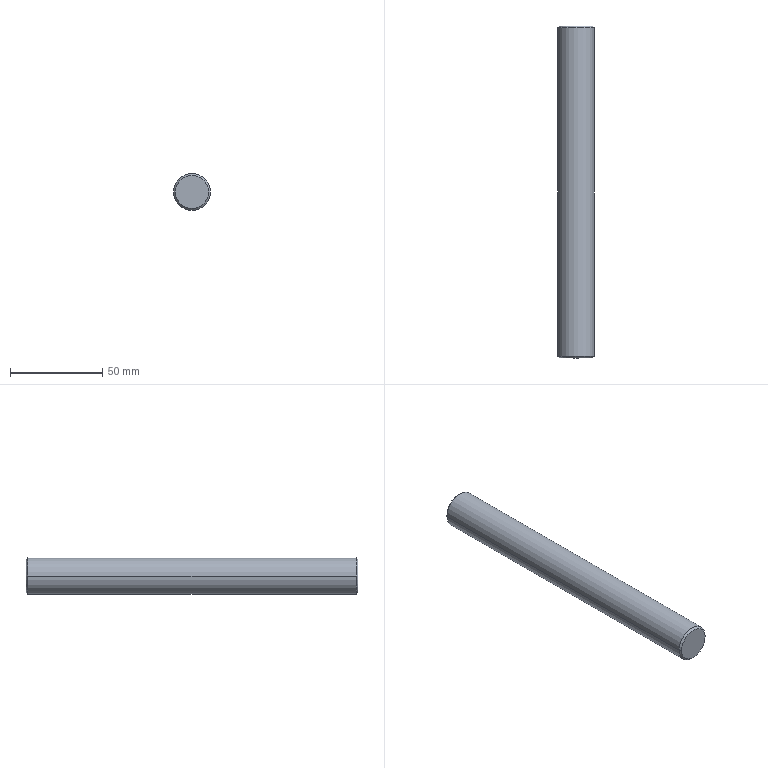Part | SolidWorks | features BaseBody 1 | 1 solid | 8 faces | box 20 x 180 x 20 mm | volume 56488 mm3 | cone 4 | cylinder 2 | plane 2 | commonest cylinder face diameters 20 x2
STEP:
#1=CARTESIAN_POINT('',(-9.,90.,0.));
#2=VERTEX_POINT('',#1);
#3=CARTESIAN_POINT('',(9.,90.,0.));
#4=VERTEX_POINT('',#3);
#5=CARTESIAN_POINT('',(0.,90.,0.));
#6=DIRECTION('',(0.,1.,0.));
#7=DIRECTION('',(-1.,0.,0.));
#8=AXIS2_PLACEMENT_3D('',#5,#6,#7);
#9=CIRCLE('',#8,9.);
#10=EDGE_CURVE('',#2,#4,#9,.T.);
#11=ORIENTED_EDGE('',*,*,#10,.F.);
#12=CARTESIAN_POINT('',(-10.,89.,0.));
#13=VERTEX_POINT('',#12);
#14=CARTESIAN_POINT('',(-10.,89.,0.));
#15=DIRECTION('',(-0.7071,-0.7071,0.));
#16=VECTOR('',#15,1000.);
#17=LINE('',#14,#16);
#18=EDGE_CURVE('',#2,#13,#17,.T.);
#19=ORIENTED_EDGE('',*,*,#18,.T.);
#20=CARTESIAN_POINT('',(10.,89.,0.));
#21=VERTEX_POINT('',#20);
#22=CARTESIAN_POINT('',(0.,89.,0.));
#23=DIRECTION('',(0.,1.,0.));
#24=DIRECTION('',(-1.,0.,0.));
#25=AXIS2_PLACEMENT_3D('',#22,#23,#24);
#26=CIRCLE('',#25,10.);
#27=EDGE_CURVE('',#13,#21,#26,.T.);
#28=ORIENTED_EDGE('',*,*,#27,.T.);
#29=CARTESIAN_POINT('',(10.,89.,0.));
#30=DIRECTION('',(0.7071,-0.7071,0.));
#31=VECTOR('',#30,1000.);
#32=LINE('',#29,#31);
#33=EDGE_CURVE('',#4,#21,#32,.T.);
#34=ORIENTED_EDGE('',*,*,#33,.F.);
#35=EDGE_LOOP('',(#11,#19,#28,#34));
#36=FACE_OUTER_BOUND('',#35,.T.);
#37=CARTESIAN_POINT('',(0.,89.,0.));
#38=DIRECTION('',(0.,-1.,0.));
#39=DIRECTION('',(1.,0.,0.));
#40=AXIS2_PLACEMENT_3D('',#37,#38,#39);
#41=CONICAL_SURFACE('',#40,10.,0.7854);
#42=ADVANCED_FACE('',(#36),#41,.T.);
#43=CARTESIAN_POINT('',(-10.,-89.,0.));
#44=VERTEX_POINT('',#43);
#45=CARTESIAN_POINT('',(10.,-89.,0.));
#46=VERTEX_POINT('',#45);
#47=CARTESIAN_POINT('',(0.,-89.,0.));
#48=DIRECTION('',(0.,1.,0.));
#49=DIRECTION('',(-1.,0.,0.));
#50=AXIS2_PLACEMENT_3D('',#47,#48,#49);
#51=CIRCLE('',#50,10.);
#52=EDGE_CURVE('',#44,#46,#51,.T.);
#53=ORIENTED_EDGE('',*,*,#52,.T.);
#54=CARTESIAN_POINT('',(10.,90.,0.));
#55=DIRECTION('',(0.,1.,0.));
#56=VECTOR('',#55,1000.);
#57=LINE('',#54,#56);
#58=EDGE_CURVE('',#46,#21,#57,.T.);
#59=ORIENTED_EDGE('',*,*,#58,.T.);
#60=ORIENTED_EDGE('',*,*,#27,.F.);
#61=CARTESIAN_POINT('',(-10.,90.,0.));
#62=DIRECTION('',(0.,1.,0.));
#63=VECTOR('',#62,1000.);
#64=LINE('',#61,#63);
#65=EDGE_CURVE('',#44,#13,#64,.T.);
#66=ORIENTED_EDGE('',*,*,#65,.F.);
#67=EDGE_LOOP('',(#53,#59,#60,#66));
#68=FACE_OUTER_BOUND('',#67,.T.);
#69=CARTESIAN_POINT('',(0.,90.,0.));
#70=DIRECTION('',(0.,1.,0.));
#71=DIRECTION('',(-1.,0.,0.));
#72=AXIS2_PLACEMENT_3D('',#69,#70,#71);
#73=CYLINDRICAL_SURFACE('',#72,10.);
#74=ADVANCED_FACE('',(#68),#73,.T.);
#75=CARTESIAN_POINT('',(-9.,-90.,0.));
#76=VERTEX_POINT('',#75);
#77=CARTESIAN_POINT('',(9.,-90.,0.));
#78=VERTEX_POINT('',#77);
#79=CARTESIAN_POINT('',(0.,-90.,0.));
#80=DIRECTION('',(0.,1.,0.));
#81=DIRECTION('',(-1.,0.,0.));
#82=AXIS2_PLACEMENT_3D('',#79,#80,#81);
#83=CIRCLE('',#82,9.);
#84=EDGE_CURVE('',#76,#78,#83,.T.);
#85=ORIENTED_EDGE('',*,*,#84,.T.);
#86=CARTESIAN_POINT('',(9.,-90.,0.));
#87=DIRECTION('',(0.7071,0.7071,0.));
#88=VECTOR('',#87,1000.);
#89=LINE('',#86,#88);
#90=EDGE_CURVE('',#78,#46,#89,.T.);
#91=ORIENTED_EDGE('',*,*,#90,.T.);
#92=ORIENTED_EDGE('',*,*,#52,.F.);
#93=CARTESIAN_POINT('',(-9.,-90.,0.));
#94=DIRECTION('',(-0.7071,0.7071,0.));
#95=VECTOR('',#94,1000.);
#96=LINE('',#93,#95);
#97=EDGE_CURVE('',#76,#44,#96,.T.);
#98=ORIENTED_EDGE('',*,*,#97,.F.);
#99=EDGE_LOOP('',(#85,#91,#92,#98));
#100=FACE_OUTER_BOUND('',#99,.T.);
#101=CARTESIAN_POINT('',(0.,-90.,0.));
#102=DIRECTION('',(0.,1.,0.));
#103=DIRECTION('',(-1.,0.,0.));
#104=AXIS2_PLACEMENT_3D('',#101,#102,#103);
#105=CONICAL_SURFACE('',#104,9.,0.7854);
#106=ADVANCED_FACE('',(#100),#105,.T.);
#107=ORIENTED_EDGE('',*,*,#90,.F.);
#108=CARTESIAN_POINT('',(0.,-90.,0.));
#109=DIRECTION('',(0.,1.,0.));
#110=DIRECTION('',(-1.,0.,0.));
#111=AXIS2_PLACEMENT_3D('',#108,#109,#110);
#112=CIRCLE('',#111,9.);
#113=EDGE_CURVE('',#78,#76,#112,.T.);
#114=ORIENTED_EDGE('',*,*,#113,.T.);
#115=ORIENTED_EDGE('',*,*,#97,.T.);
#116=CARTESIAN_POINT('',(0.,-89.,0.));
#117=DIRECTION('',(0.,1.,0.));
#118=DIRECTION('',(-1.,0.,0.));
#119=AXIS2_PLACEMENT_3D('',#116,#117,#118);
#120=CIRCLE('',#119,10.);
#121=EDGE_CURVE('',#46,#44,#120,.T.);
#122=ORIENTED_EDGE('',*,*,#121,.F.);
#123=EDGE_LOOP('',(#107,#114,#115,#122));
#124=FACE_OUTER_BOUND('',#123,.T.);
#125=CARTESIAN_POINT('',(0.,-90.,0.));
#126=DIRECTION('',(0.,1.,0.));
#127=DIRECTION('',(-1.,0.,0.));
#128=AXIS2_PLACEMENT_3D('',#125,#126,#127);
#129=CONICAL_SURFACE('',#128,9.,0.7854);
#130=ADVANCED_FACE('',(#124),#129,.T.);
#131=ORIENTED_EDGE('',*,*,#58,.F.);
#132=ORIENTED_EDGE('',*,*,#121,.T.);
#133=ORIENTED_EDGE('',*,*,#65,.T.);
#134=CARTESIAN_POINT('',(0.,89.,0.));
#135=DIRECTION('',(0.,1.,0.));
#136=DIRECTION('',(-1.,0.,0.));
#137=AXIS2_PLACEMENT_3D('',#134,#135,#136);
#138=CIRCLE('',#137,10.);
#139=EDGE_CURVE('',#21,#13,#138,.T.);
#140=ORIENTED_EDGE('',*,*,#139,.F.);
#141=EDGE_LOOP('',(#131,#132,#133,#140));
#142=FACE_OUTER_BOUND('',#141,.T.);
#143=CARTESIAN_POINT('',(0.,90.,0.));
#144=DIRECTION('',(0.,1.,0.));
#145=DIRECTION('',(-1.,0.,0.));
#146=AXIS2_PLACEMENT_3D('',#143,#144,#145);
#147=CYLINDRICAL_SURFACE('',#146,10.);
#148=ADVANCED_FACE('',(#142),#147,.T.);
#149=ORIENTED_EDGE('',*,*,#18,.F.);
#150=CARTESIAN_POINT('',(0.,90.,0.));
#151=DIRECTION('',(0.,1.,0.));
#152=DIRECTION('',(-1.,0.,0.));
#153=AXIS2_PLACEMENT_3D('',#150,#151,#152);
#154=CIRCLE('',#153,9.);
#155=EDGE_CURVE('',#4,#2,#154,.T.);
#156=ORIENTED_EDGE('',*,*,#155,.F.);
#157=ORIENTED_EDGE('',*,*,#33,.T.);
#158=ORIENTED_EDGE('',*,*,#139,.T.);
#159=EDGE_LOOP('',(#149,#156,#157,#158));
#160=FACE_OUTER_BOUND('',#159,.T.);
#161=CARTESIAN_POINT('',(0.,89.,0.));
#162=DIRECTION('',(0.,-1.,0.));
#163=DIRECTION('',(1.,0.,0.));
#164=AXIS2_PLACEMENT_3D('',#161,#162,#163);
#165=CONICAL_SURFACE('',#164,10.,0.7854);
#166=ADVANCED_FACE('',(#160),#165,.T.);
#167=ORIENTED_EDGE('',*,*,#155,.T.);
#168=ORIENTED_EDGE('',*,*,#10,.T.);
#169=EDGE_LOOP('',(#167,#168));
#170=FACE_OUTER_BOUND('',#169,.T.);
#171=CARTESIAN_POINT('',(0.,90.,0.));
#172=DIRECTION('',(0.,-1.,0.));
#173=DIRECTION('',(1.,0.,0.));
#174=AXIS2_PLACEMENT_3D('',#171,#172,#173);
#175=PLANE('',#174);
#176=ADVANCED_FACE('',(#170),#175,.F.);
#177=ORIENTED_EDGE('',*,*,#84,.F.);
#178=ORIENTED_EDGE('',*,*,#113,.F.);
#179=EDGE_LOOP('',(#177,#178));
#180=FACE_OUTER_BOUND('',#179,.T.);
#181=CARTESIAN_POINT('',(9.,-90.,0.));
#182=DIRECTION('',(0.,1.,0.));
#183=DIRECTION('',(-1.,0.,0.));
#184=AXIS2_PLACEMENT_3D('',#181,#182,#183);
#185=PLANE('',#184);
#186=ADVANCED_FACE('',(#180),#185,.F.);
#187=CLOSED_SHELL('',(#42,#74,#106,#130,#148,#166,#176,#186));
#188=MANIFOLD_SOLID_BREP('',#187);
#189=CARTESIAN_POINT('',(0.,0.,0.));
#190=DIRECTION('',(0.,0.,1.));
#191=DIRECTION('',(1.,0.,0.));
#192=AXIS2_PLACEMENT_3D('',#189,#190,#191);
#193=(LENGTH_UNIT()NAMED_UNIT(*)SI_UNIT(.MILLI.,.METRE.));
#194=UNCERTAINTY_MEASURE_WITH_UNIT(LENGTH_MEASURE(0.00001),#193,'','');
#195=(NAMED_UNIT(*)PLANE_ANGLE_UNIT()SI_UNIT($,.RADIAN.));
#196=(NAMED_UNIT(*)SI_UNIT($,.STERADIAN.)SOLID_ANGLE_UNIT());
#197=(GEOMETRIC_REPRESENTATION_CONTEXT(3)GLOBAL_UNCERTAINTY_ASSIGNED_CONTEXT((#194))GLOBAL_UNIT_ASSIGNED_CONTEXT((#193,#195,#196))REPRESENTATION_CONTEXT('',''));
#198=ADVANCED_BREP_SHAPE_REPRESENTATION('',(#188,#192),#197);